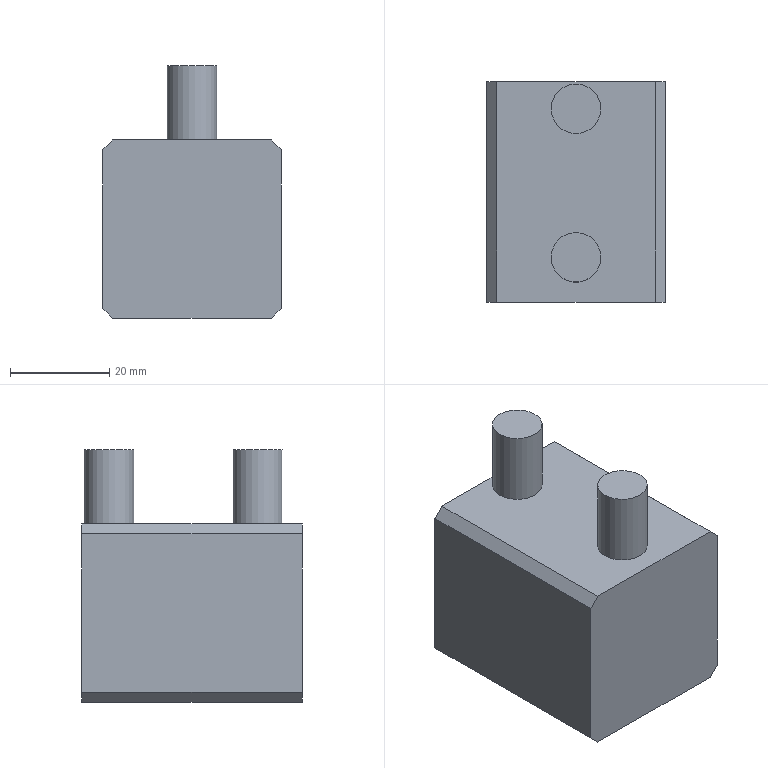Part | NX | features solid 2 | 1 solid | 14 faces | box 36 x 44.5 x 51 mm | volume 59672 mm3 | plane 12 | cylinder 2 | commonest cylinder face diameters 10 x2
STEP:
#1=CARTESIAN_POINT('',(450.131,101.387,166.));
#2=VERTEX_POINT('',#1);
#3=CARTESIAN_POINT('',(418.131,101.387,166.));
#4=VERTEX_POINT('',#3);
#5=CARTESIAN_POINT('',(461.131,101.387,166.));
#6=DIRECTION('',(-1.,0.,0.));
#7=VECTOR('',#6,1000.);
#8=LINE('',#5,#7);
#9=EDGE_CURVE('',#2,#4,#8,.T.);
#10=ORIENTED_EDGE('',*,*,#9,.T.);
#11=CARTESIAN_POINT('',(416.131,101.387,168.));
#12=VERTEX_POINT('',#11);
#13=CARTESIAN_POINT('',(416.131,101.387,168.));
#14=DIRECTION('',(-0.7071,0.,0.7071));
#15=VECTOR('',#14,1000.);
#16=LINE('',#13,#15);
#17=EDGE_CURVE('',#4,#12,#16,.T.);
#18=ORIENTED_EDGE('',*,*,#17,.T.);
#19=CARTESIAN_POINT('',(416.131,101.387,200.));
#20=VERTEX_POINT('',#19);
#21=CARTESIAN_POINT('',(416.131,101.387,166.));
#22=DIRECTION('',(0.,0.,1.));
#23=VECTOR('',#22,1000.);
#24=LINE('',#21,#23);
#25=EDGE_CURVE('',#12,#20,#24,.T.);
#26=ORIENTED_EDGE('',*,*,#25,.T.);
#27=CARTESIAN_POINT('',(418.131,101.387,202.));
#28=VERTEX_POINT('',#27);
#29=CARTESIAN_POINT('',(416.131,101.387,200.));
#30=DIRECTION('',(-0.7071,0.,-0.7071));
#31=VECTOR('',#30,1000.);
#32=LINE('',#29,#31);
#33=EDGE_CURVE('',#20,#28,#32,.F.);
#34=ORIENTED_EDGE('',*,*,#33,.T.);
#35=CARTESIAN_POINT('',(450.131,101.387,202.));
#36=VERTEX_POINT('',#35);
#37=CARTESIAN_POINT('',(461.131,101.387,202.));
#38=DIRECTION('',(-1.,0.,0.));
#39=VECTOR('',#38,1000.);
#40=LINE('',#37,#39);
#41=EDGE_CURVE('',#36,#28,#40,.T.);
#42=ORIENTED_EDGE('',*,*,#41,.F.);
#43=CARTESIAN_POINT('',(452.131,101.387,200.));
#44=VERTEX_POINT('',#43);
#45=CARTESIAN_POINT('',(450.131,101.387,202.));
#46=DIRECTION('',(-0.7071,0.,0.7071));
#47=VECTOR('',#46,1000.);
#48=LINE('',#45,#47);
#49=EDGE_CURVE('',#44,#36,#48,.T.);
#50=ORIENTED_EDGE('',*,*,#49,.F.);
#51=CARTESIAN_POINT('',(452.131,101.387,168.));
#52=VERTEX_POINT('',#51);
#53=CARTESIAN_POINT('',(452.131,101.387,166.));
#54=DIRECTION('',(0.,0.,-1.));
#55=VECTOR('',#54,1000.);
#56=LINE('',#53,#55);
#57=EDGE_CURVE('',#52,#44,#56,.F.);
#58=ORIENTED_EDGE('',*,*,#57,.F.);
#59=CARTESIAN_POINT('',(452.131,101.387,168.));
#60=DIRECTION('',(-0.7071,0.,-0.7071));
#61=VECTOR('',#60,1000.);
#62=LINE('',#59,#61);
#63=EDGE_CURVE('',#2,#52,#62,.F.);
#64=ORIENTED_EDGE('',*,*,#63,.F.);
#65=EDGE_LOOP('',(#10,#18,#26,#34,#42,#50,#58,#64));
#66=FACE_BOUND('',#65,.T.);
#67=CARTESIAN_POINT('',(461.131,101.387,166.));
#68=DIRECTION('',(0.,1.,0.));
#69=DIRECTION('',(-1.,0.,0.));
#70=AXIS2_PLACEMENT_3D('',#67,#68,#69);
#71=PLANE('',#70);
#72=ADVANCED_FACE('',(#66),#71,.T.);
#73=ORIENTED_EDGE('',*,*,#25,.F.);
#74=CARTESIAN_POINT('',(416.131,56.887,168.));
#75=VERTEX_POINT('',#74);
#76=CARTESIAN_POINT('',(416.131,56.887,168.));
#77=DIRECTION('',(0.,1.,0.));
#78=VECTOR('',#77,1000.);
#79=LINE('',#76,#78);
#80=EDGE_CURVE('',#12,#75,#79,.F.);
#81=ORIENTED_EDGE('',*,*,#80,.T.);
#82=CARTESIAN_POINT('',(416.131,56.887,200.));
#83=VERTEX_POINT('',#82);
#84=CARTESIAN_POINT('',(416.131,56.887,166.));
#85=DIRECTION('',(0.,0.,-1.));
#86=VECTOR('',#85,1000.);
#87=LINE('',#84,#86);
#88=EDGE_CURVE('',#75,#83,#87,.F.);
#89=ORIENTED_EDGE('',*,*,#88,.T.);
#90=CARTESIAN_POINT('',(416.131,101.387,200.));
#91=DIRECTION('',(0.,-1.,0.));
#92=VECTOR('',#91,1000.);
#93=LINE('',#90,#92);
#94=EDGE_CURVE('',#83,#20,#93,.F.);
#95=ORIENTED_EDGE('',*,*,#94,.T.);
#96=EDGE_LOOP('',(#73,#81,#89,#95));
#97=FACE_BOUND('',#96,.T.);
#98=CARTESIAN_POINT('',(416.131,101.387,166.));
#99=DIRECTION('',(-1.,0.,0.));
#100=DIRECTION('',(0.,-1.,0.));
#101=AXIS2_PLACEMENT_3D('',#98,#99,#100);
#102=PLANE('',#101);
#103=ADVANCED_FACE('',(#97),#102,.T.);
#104=ORIENTED_EDGE('',*,*,#88,.F.);
#105=CARTESIAN_POINT('',(418.131,56.887,166.));
#106=VERTEX_POINT('',#105);
#107=CARTESIAN_POINT('',(416.131,56.887,168.));
#108=DIRECTION('',(-0.7071,0.,0.7071));
#109=VECTOR('',#108,1000.);
#110=LINE('',#107,#109);
#111=EDGE_CURVE('',#75,#106,#110,.F.);
#112=ORIENTED_EDGE('',*,*,#111,.T.);
#113=CARTESIAN_POINT('',(450.131,56.887,166.));
#114=VERTEX_POINT('',#113);
#115=CARTESIAN_POINT('',(461.131,56.887,166.));
#116=DIRECTION('',(-1.,0.,0.));
#117=VECTOR('',#116,1000.);
#118=LINE('',#115,#117);
#119=EDGE_CURVE('',#114,#106,#118,.T.);
#120=ORIENTED_EDGE('',*,*,#119,.F.);
#121=CARTESIAN_POINT('',(452.131,56.887,168.));
#122=VERTEX_POINT('',#121);
#123=CARTESIAN_POINT('',(452.131,56.887,168.));
#124=DIRECTION('',(-0.7071,0.,-0.7071));
#125=VECTOR('',#124,1000.);
#126=LINE('',#123,#125);
#127=EDGE_CURVE('',#122,#114,#126,.T.);
#128=ORIENTED_EDGE('',*,*,#127,.F.);
#129=CARTESIAN_POINT('',(452.131,56.887,200.));
#130=VERTEX_POINT('',#129);
#131=CARTESIAN_POINT('',(452.131,56.887,166.));
#132=DIRECTION('',(0.,0.,1.));
#133=VECTOR('',#132,1000.);
#134=LINE('',#131,#133);
#135=EDGE_CURVE('',#122,#130,#134,.T.);
#136=ORIENTED_EDGE('',*,*,#135,.T.);
#137=CARTESIAN_POINT('',(450.131,56.887,202.));
#138=VERTEX_POINT('',#137);
#139=CARTESIAN_POINT('',(450.131,56.887,202.));
#140=DIRECTION('',(-0.7071,0.,0.7071));
#141=VECTOR('',#140,1000.);
#142=LINE('',#139,#141);
#143=EDGE_CURVE('',#138,#130,#142,.F.);
#144=ORIENTED_EDGE('',*,*,#143,.F.);
#145=CARTESIAN_POINT('',(418.131,56.887,202.));
#146=VERTEX_POINT('',#145);
#147=CARTESIAN_POINT('',(461.131,56.887,202.));
#148=DIRECTION('',(-1.,0.,0.));
#149=VECTOR('',#148,1000.);
#150=LINE('',#147,#149);
#151=EDGE_CURVE('',#138,#146,#150,.T.);
#152=ORIENTED_EDGE('',*,*,#151,.T.);
#153=CARTESIAN_POINT('',(416.131,56.887,200.));
#154=DIRECTION('',(-0.7071,0.,-0.7071));
#155=VECTOR('',#154,1000.);
#156=LINE('',#153,#155);
#157=EDGE_CURVE('',#146,#83,#156,.T.);
#158=ORIENTED_EDGE('',*,*,#157,.T.);
#159=EDGE_LOOP('',(#104,#112,#120,#128,#136,#144,#152,#158));
#160=FACE_BOUND('',#159,.T.);
#161=CARTESIAN_POINT('',(461.131,56.887,166.));
#162=DIRECTION('',(0.,1.,0.));
#163=DIRECTION('',(-1.,0.,0.));
#164=AXIS2_PLACEMENT_3D('',#161,#162,#163);
#165=PLANE('',#164);
#166=ADVANCED_FACE('',(#160),#165,.F.);
#167=ORIENTED_EDGE('',*,*,#135,.F.);
#168=CARTESIAN_POINT('',(452.131,56.887,168.));
#169=DIRECTION('',(0.,-1.,0.));
#170=VECTOR('',#169,1000.);
#171=LINE('',#168,#170);
#172=EDGE_CURVE('',#52,#122,#171,.T.);
#173=ORIENTED_EDGE('',*,*,#172,.F.);
#174=ORIENTED_EDGE('',*,*,#57,.T.);
#175=CARTESIAN_POINT('',(452.131,101.387,200.));
#176=DIRECTION('',(0.,1.,0.));
#177=VECTOR('',#176,1000.);
#178=LINE('',#175,#177);
#179=EDGE_CURVE('',#130,#44,#178,.T.);
#180=ORIENTED_EDGE('',*,*,#179,.F.);
#181=EDGE_LOOP('',(#167,#173,#174,#180));
#182=FACE_BOUND('',#181,.T.);
#183=CARTESIAN_POINT('',(452.131,101.387,166.));
#184=DIRECTION('',(-1.,0.,0.));
#185=DIRECTION('',(0.,-1.,0.));
#186=AXIS2_PLACEMENT_3D('',#183,#184,#185);
#187=PLANE('',#186);
#188=ADVANCED_FACE('',(#182),#187,.F.);
#189=ORIENTED_EDGE('',*,*,#41,.T.);
#190=CARTESIAN_POINT('',(418.131,101.387,202.));
#191=DIRECTION('',(0.,-1.,0.));
#192=VECTOR('',#191,1000.);
#193=LINE('',#190,#192);
#194=EDGE_CURVE('',#28,#146,#193,.T.);
#195=ORIENTED_EDGE('',*,*,#194,.T.);
#196=ORIENTED_EDGE('',*,*,#151,.F.);
#197=CARTESIAN_POINT('',(450.131,101.387,202.));
#198=DIRECTION('',(0.,1.,0.));
#199=VECTOR('',#198,1000.);
#200=LINE('',#197,#199);
#201=EDGE_CURVE('',#36,#138,#200,.F.);
#202=ORIENTED_EDGE('',*,*,#201,.F.);
#203=EDGE_LOOP('',(#189,#195,#196,#202));
#204=FACE_BOUND('',#203,.T.);
#205=CARTESIAN_POINT('',(429.131,95.887,202.));
#206=VERTEX_POINT('',#205);
#207=CARTESIAN_POINT('',(434.131,95.887,202.));
#208=DIRECTION('',(0.,0.,1.));
#209=DIRECTION('',(-1.,0.,0.));
#210=AXIS2_PLACEMENT_3D('',#207,#208,#209);
#211=CIRCLE('',#210,5.);
#212=EDGE_CURVE('',#206,#206,#211,.F.);
#213=ORIENTED_EDGE('',*,*,#212,.T.);
#214=EDGE_LOOP('',(#213));
#215=FACE_BOUND('',#214,.T.);
#216=CARTESIAN_POINT('',(429.131,65.887,202.));
#217=VERTEX_POINT('',#216);
#218=CARTESIAN_POINT('',(434.131,65.887,202.));
#219=DIRECTION('',(0.,0.,1.));
#220=DIRECTION('',(-1.,0.,0.));
#221=AXIS2_PLACEMENT_3D('',#218,#219,#220);
#222=CIRCLE('',#221,5.);
#223=EDGE_CURVE('',#217,#217,#222,.F.);
#224=ORIENTED_EDGE('',*,*,#223,.T.);
#225=EDGE_LOOP('',(#224));
#226=FACE_BOUND('',#225,.T.);
#227=CARTESIAN_POINT('',(461.131,101.387,202.));
#228=DIRECTION('',(0.,0.,-1.));
#229=DIRECTION('',(-1.,0.,0.));
#230=AXIS2_PLACEMENT_3D('',#227,#228,#229);
#231=PLANE('',#230);
#232=ADVANCED_FACE('',(#204,#215,#226),#231,.F.);
#233=ORIENTED_EDGE('',*,*,#119,.T.);
#234=CARTESIAN_POINT('',(418.131,101.387,166.));
#235=DIRECTION('',(0.,1.,0.));
#236=VECTOR('',#235,1000.);
#237=LINE('',#234,#236);
#238=EDGE_CURVE('',#106,#4,#237,.T.);
#239=ORIENTED_EDGE('',*,*,#238,.T.);
#240=ORIENTED_EDGE('',*,*,#9,.F.);
#241=CARTESIAN_POINT('',(450.131,101.387,166.));
#242=DIRECTION('',(0.,1.,0.));
#243=VECTOR('',#242,1000.);
#244=LINE('',#241,#243);
#245=EDGE_CURVE('',#114,#2,#244,.T.);
#246=ORIENTED_EDGE('',*,*,#245,.F.);
#247=EDGE_LOOP('',(#233,#239,#240,#246));
#248=FACE_BOUND('',#247,.T.);
#249=CARTESIAN_POINT('',(461.131,101.387,166.));
#250=DIRECTION('',(0.,0.,-1.));
#251=DIRECTION('',(-1.,0.,0.));
#252=AXIS2_PLACEMENT_3D('',#249,#250,#251);
#253=PLANE('',#252);
#254=ADVANCED_FACE('',(#248),#253,.T.);
#255=CARTESIAN_POINT('',(439.131,65.887,217.));
#256=VERTEX_POINT('',#255);
#257=CARTESIAN_POINT('',(434.131,65.887,217.));
#258=DIRECTION('',(0.,0.,1.));
#259=DIRECTION('',(1.,0.,0.));
#260=AXIS2_PLACEMENT_3D('',#257,#258,#259);
#261=CIRCLE('',#260,5.);
#262=EDGE_CURVE('',#256,#256,#261,.F.);
#263=ORIENTED_EDGE('',*,*,#262,.F.);
#264=EDGE_LOOP('',(#263));
#265=FACE_BOUND('',#264,.T.);
#266=CARTESIAN_POINT('',(434.131,65.887,217.));
#267=DIRECTION('',(0.,0.,1.));
#268=DIRECTION('',(1.,0.,0.));
#269=AXIS2_PLACEMENT_3D('',#266,#267,#268);
#270=PLANE('',#269);
#271=ADVANCED_FACE('',(#265),#270,.T.);
#272=ORIENTED_EDGE('',*,*,#262,.T.);
#273=EDGE_LOOP('',(#272));
#274=FACE_BOUND('',#273,.T.);
#275=ORIENTED_EDGE('',*,*,#223,.F.);
#276=EDGE_LOOP('',(#275));
#277=FACE_BOUND('',#276,.T.);
#278=CARTESIAN_POINT('',(434.131,65.887,202.));
#279=DIRECTION('',(0.,0.,1.));
#280=DIRECTION('',(1.,0.,0.));
#281=AXIS2_PLACEMENT_3D('',#278,#279,#280);
#282=CYLINDRICAL_SURFACE('',#281,5.);
#283=ADVANCED_FACE('',(#274,#277),#282,.T.);
#284=CARTESIAN_POINT('',(439.131,95.887,217.));
#285=VERTEX_POINT('',#284);
#286=CARTESIAN_POINT('',(434.131,95.887,217.));
#287=DIRECTION('',(0.,0.,1.));
#288=DIRECTION('',(1.,0.,0.));
#289=AXIS2_PLACEMENT_3D('',#286,#287,#288);
#290=CIRCLE('',#289,5.);
#291=EDGE_CURVE('',#285,#285,#290,.F.);
#292=ORIENTED_EDGE('',*,*,#291,.F.);
#293=EDGE_LOOP('',(#292));
#294=FACE_BOUND('',#293,.T.);
#295=CARTESIAN_POINT('',(434.131,95.887,217.));
#296=DIRECTION('',(0.,0.,1.));
#297=DIRECTION('',(1.,0.,0.));
#298=AXIS2_PLACEMENT_3D('',#295,#296,#297);
#299=PLANE('',#298);
#300=ADVANCED_FACE('',(#294),#299,.T.);
#301=ORIENTED_EDGE('',*,*,#291,.T.);
#302=EDGE_LOOP('',(#301));
#303=FACE_BOUND('',#302,.T.);
#304=ORIENTED_EDGE('',*,*,#212,.F.);
#305=EDGE_LOOP('',(#304));
#306=FACE_BOUND('',#305,.T.);
#307=CARTESIAN_POINT('',(434.131,95.887,202.));
#308=DIRECTION('',(0.,0.,1.));
#309=DIRECTION('',(1.,0.,0.));
#310=AXIS2_PLACEMENT_3D('',#307,#308,#309);
#311=CYLINDRICAL_SURFACE('',#310,5.);
#312=ADVANCED_FACE('',(#303,#306),#311,.T.);
#313=ORIENTED_EDGE('',*,*,#49,.T.);
#314=ORIENTED_EDGE('',*,*,#201,.T.);
#315=ORIENTED_EDGE('',*,*,#143,.T.);
#316=ORIENTED_EDGE('',*,*,#179,.T.);
#317=EDGE_LOOP('',(#313,#314,#315,#316));
#318=FACE_BOUND('',#317,.T.);
#319=CARTESIAN_POINT('',(450.131,101.387,202.));
#320=DIRECTION('',(-0.7071,0.,-0.7071));
#321=DIRECTION('',(-0.7071,0.,0.7071));
#322=AXIS2_PLACEMENT_3D('',#319,#320,#321);
#323=PLANE('',#322);
#324=ADVANCED_FACE('',(#318),#323,.F.);
#325=ORIENTED_EDGE('',*,*,#63,.T.);
#326=ORIENTED_EDGE('',*,*,#172,.T.);
#327=ORIENTED_EDGE('',*,*,#127,.T.);
#328=ORIENTED_EDGE('',*,*,#245,.T.);
#329=EDGE_LOOP('',(#325,#326,#327,#328));
#330=FACE_BOUND('',#329,.T.);
#331=CARTESIAN_POINT('',(452.131,101.387,168.));
#332=DIRECTION('',(0.7071,0.,-0.7071));
#333=DIRECTION('',(-0.7071,0.,-0.7071));
#334=AXIS2_PLACEMENT_3D('',#331,#332,#333);
#335=PLANE('',#334);
#336=ADVANCED_FACE('',(#330),#335,.T.);
#337=ORIENTED_EDGE('',*,*,#17,.F.);
#338=ORIENTED_EDGE('',*,*,#238,.F.);
#339=ORIENTED_EDGE('',*,*,#111,.F.);
#340=ORIENTED_EDGE('',*,*,#80,.F.);
#341=EDGE_LOOP('',(#337,#338,#339,#340));
#342=FACE_BOUND('',#341,.T.);
#343=CARTESIAN_POINT('',(416.131,101.387,168.));
#344=DIRECTION('',(0.7071,0.,0.7071));
#345=DIRECTION('',(0.7071,0.,-0.7071));
#346=AXIS2_PLACEMENT_3D('',#343,#344,#345);
#347=PLANE('',#346);
#348=ADVANCED_FACE('',(#342),#347,.F.);
#349=ORIENTED_EDGE('',*,*,#157,.F.);
#350=ORIENTED_EDGE('',*,*,#194,.F.);
#351=ORIENTED_EDGE('',*,*,#33,.F.);
#352=ORIENTED_EDGE('',*,*,#94,.F.);
#353=EDGE_LOOP('',(#349,#350,#351,#352));
#354=FACE_BOUND('',#353,.T.);
#355=CARTESIAN_POINT('',(416.131,101.387,200.));
#356=DIRECTION('',(-0.7071,0.,0.7071));
#357=DIRECTION('',(0.7071,0.,0.7071));
#358=AXIS2_PLACEMENT_3D('',#355,#356,#357);
#359=PLANE('',#358);
#360=ADVANCED_FACE('',(#354),#359,.T.);
#361=CLOSED_SHELL('',(#72,#103,#166,#188,#232,#254,#271,#283,#300,#312,#324,#336,#348,#360));
#362=MANIFOLD_SOLID_BREP('',#361);
#363=(LENGTH_UNIT()NAMED_UNIT(*)SI_UNIT(.MILLI.,.METRE.));
#364=UNCERTAINTY_MEASURE_WITH_UNIT(LENGTH_MEASURE(0.00001),#363,'','');
#365=(NAMED_UNIT(*)PLANE_ANGLE_UNIT()SI_UNIT($,.RADIAN.));
#366=(NAMED_UNIT(*)SI_UNIT($,.STERADIAN.)SOLID_ANGLE_UNIT());
#367=(GEOMETRIC_REPRESENTATION_CONTEXT(3)GLOBAL_UNCERTAINTY_ASSIGNED_CONTEXT((#364))GLOBAL_UNIT_ASSIGNED_CONTEXT((#363,#365,#366))REPRESENTATION_CONTEXT('',''));
#368=ADVANCED_BREP_SHAPE_REPRESENTATION('',(#362),#367);